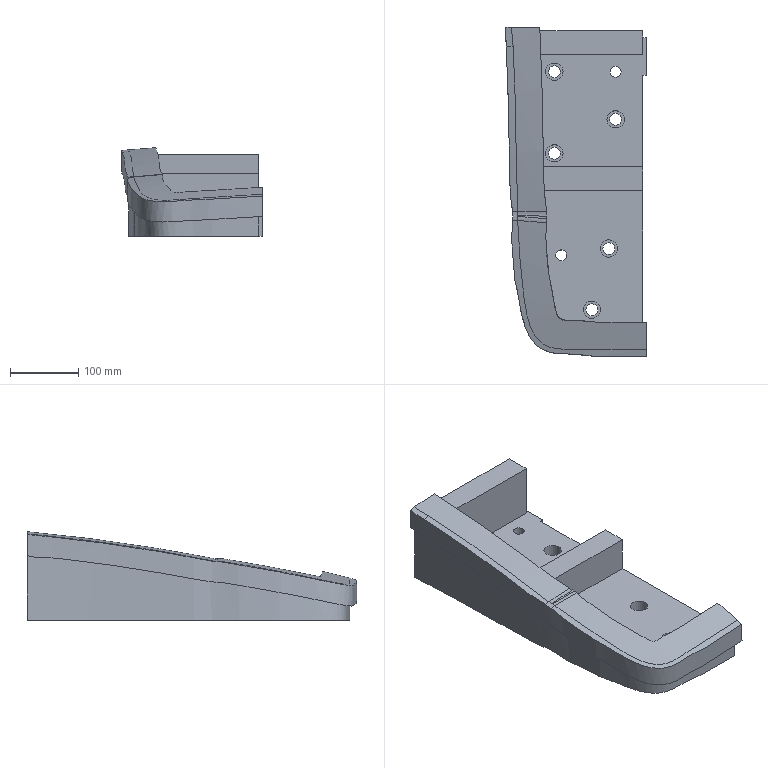Part | NX | features solid 2 | 1 solid | 50 faces | box 206.452 x 483.782 x 130.09 mm | volume 5862342 mm3 | plane 20 | spline 18 | cylinder 12 | commonest cylinder face diameters 17.5 x5 25.5 x5 16 x2